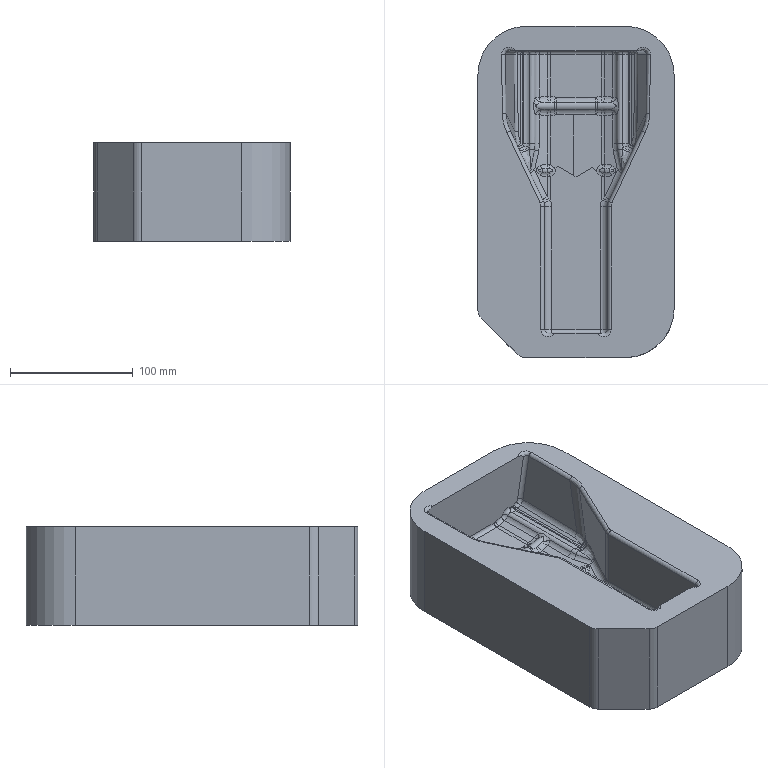CAM job | NX | 3-axis milling | part box 160 x 270 x 80 mm | stock box 160 x 270 x 80 mm
Tools:
number,name,description,diameter,corner_radius,flute_length,length,flutes
0,D25R5,Milling Tool-5 Parameters,25.0,5.0,50.0,75.0,2
0,D16R0.8,Milling Tool-5 Parameters,16.0,0.8,50.0,75.0,2
0,D8,Milling Tool-5 Parameters,8.0,0.0,50.0,75.0,2
0,D6,Milling Tool-5 Parameters,6.0,0.0,50.0,75.0,2
0,D6R3,Milling Tool-Ball Mill,6.0,3.0,70.0,75.0,2
Operations:
program,operation,operation_type,tool,method,geometry_group,spindle_rpm,surface_speed,feed_per_tooth,feed_cut,feed_plunge,cut_length_mm,path_length_mm,cut_time_min,machine_time_min
NC_PROGRAM,CAVITY_MILL,CavityMilling,D25R5,METHOD,WORKPIECE,1200.0,94.0,0.8333,2000.0,100.0,241099.193,258085.137,120.55,122.248
NC_PROGRAM,ZLEVEL_PROFILE,ZLevelMilling,D16R0.8,METHOD,WORKPIECE,2000.0,100.0,0.5,2000.0,100.0,154162.964,155234.283,77.082,77.189
NC_PROGRAM,ZLEVEL_CORNER,ZLevelMilling,D6,METHOD,WORKPIECE,0.0,0.0,0.0,1500.0,100.0,31435.498,45870.096,20.957,22.401
NC_PROGRAM,ZLEVEL_PROFILE_1,ZLevelMilling,D8,METHOD,WORKPIECE,2800.0,70.0,0.2679,1500.0,100.0,189243.028,195948.92,126.162,126.833
NC_PROGRAM,FIXED_CONTOUR,SurfaceContour,D8,METHOD,WORKPIECE,2800.0,70.0,0.2679,1500.0,100.0,146431.5,146498.7,97.621,97.628
NC_PROGRAM,FIXED_CONTOUR_COPY,SurfaceContour,D6R3,METHOD,WORKPIECE,3714.0,70.0,0.2019,1500.0,100.0,112276.387,113584.364,74.851,74.982